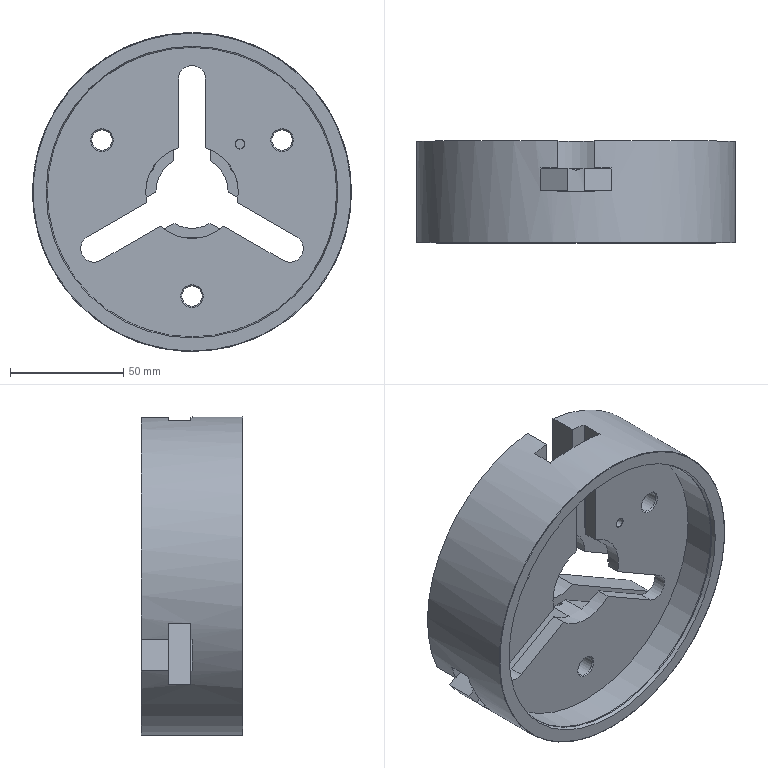NC program | NX | posted with a generic post | part box 141 x 45 x 141 mm
Whole program:
N10 G17 G21 G94 G90
(DRILLING_1 , TOOL : C20)
N12 T08 M6
N14 G54
N16 G17 G0 G90 X0. Y-22. S1300 M3
N18 G43 Z100. H8
N20 G94 G81 G98 Z-3. F300. R3.
N22 X19.053 Y11.
N24 X-19.053
N26 G80
N28 G0 X-19.053 Y11. Z100.
(DRILLING_1_COPY , TOOL : C20)
N30 X0. Y-46.
N32 G81 Z-8. F300. R3.
N34 X-39.837 Y23.
N36 X39.837
N38 G80
N40 G0 X39.837 Y23. Z100.
(PLANAR_MILL_2 , TOOL : C20)
N42 X82.373 Y4.581 S5000
N44 Z-2.
N46 G1 Z-3. F2000.
N48 X79.671 Y4.661
N50 G3 X72.469 Y-2.13 R7.
N52 G2 X-2.13 Y-72.469 R72.5
N54 X72.469 Y-2.13 R-72.5
N56 G3 X79.26 Y-9.333 R7.
N58 G1 X81.961 Y-9.413
N60 Z-2.
N62 G0 Z100.
N64 M5
N66 M2